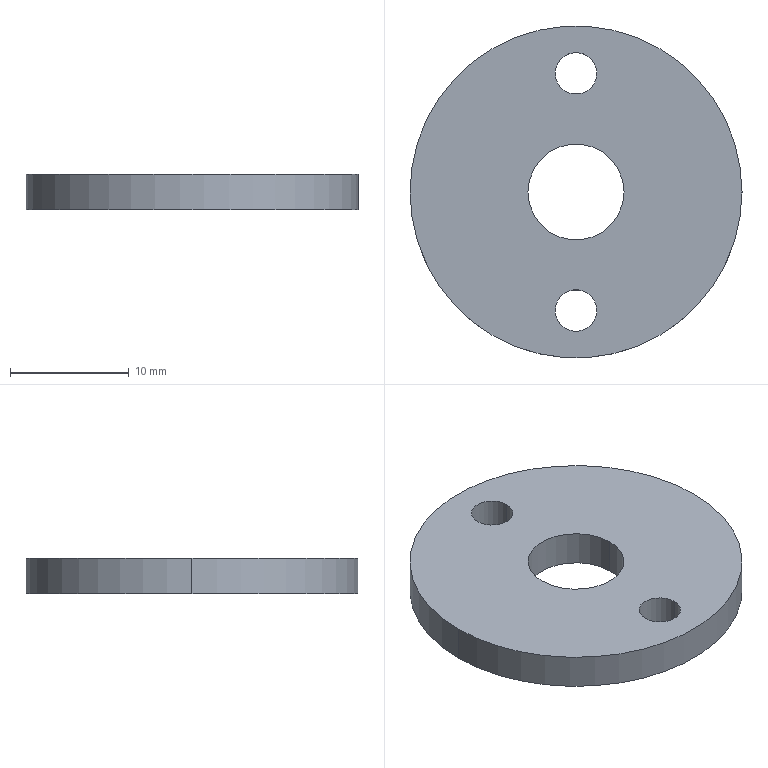Part | STEP file | BU-A19-1 | 1 solid | 10 faces | box 28 x 28 x 3 mm | volume 1635 mm3 | cylinder 8 | plane 2 | commonest cylinder face diameters 3.5 x4 8.1 x2 28 x2
STEP:
#1=CARTESIAN_POINT('',(0.,0.,0.));
#2=DIRECTION('',(0.,0.,1.));
#3=DIRECTION('',(1.,0.,0.));
#4=AXIS2_PLACEMENT_3D('',#1,#2,#3);
#5=CARTESIAN_POINT('',(-1.75,-10.,3.));
#6=VERTEX_POINT('',#5);
#7=CARTESIAN_POINT('',(-1.75,-10.,0.));
#8=VERTEX_POINT('',#7);
#9=CARTESIAN_POINT('',(-1.75,-10.,3.));
#10=DIRECTION('',(0.,0.,-1.));
#11=VECTOR('',#10,1.);
#12=LINE('',#9,#11);
#13=CARTESIAN_POINT('',(0.,-10.,3.));
#14=DIRECTION('',(0.,0.,-1.));
#15=DIRECTION('',(-1.,0.,0.));
#16=AXIS2_PLACEMENT_3D('',#13,#14,#15);
#17=CYLINDRICAL_SURFACE('',#16,1.75);
#18=CARTESIAN_POINT('',(6.283,0.));
#19=DIRECTION('',(0.,1.));
#20=VECTOR('',#19,1.);
#21=LINE('',#18,#20);
#22=(GEOMETRIC_REPRESENTATION_CONTEXT(2)PARAMETRIC_REPRESENTATION_CONTEXT()REPRESENTATION_CONTEXT('',''));
#23=DEFINITIONAL_REPRESENTATION('',(#21),#22);
#24=PCURVE('',#17,#23);
#25=CARTESIAN_POINT('',(0.,-10.,3.));
#26=DIRECTION('',(0.,0.,-1.));
#27=DIRECTION('',(-1.,0.,0.));
#28=AXIS2_PLACEMENT_3D('',#25,#26,#27);
#29=CYLINDRICAL_SURFACE('',#28,1.75);
#30=CARTESIAN_POINT('',(0.,0.));
#31=DIRECTION('',(0.,1.));
#32=VECTOR('',#31,1.);
#33=LINE('',#30,#32);
#34=(GEOMETRIC_REPRESENTATION_CONTEXT(2)PARAMETRIC_REPRESENTATION_CONTEXT()REPRESENTATION_CONTEXT('',''));
#35=DEFINITIONAL_REPRESENTATION('',(#33),#34);
#36=PCURVE('',#29,#35);
#37=SURFACE_CURVE('',#12,(#24,#36),.PCURVE_S1.);
#38=EDGE_CURVE('',#6,#8,#37,.T.);
#39=ORIENTED_EDGE('',*,*,#38,.T.);
#40=CARTESIAN_POINT('',(1.75,-10.,0.));
#41=VERTEX_POINT('',#40);
#42=CARTESIAN_POINT('',(0.,-10.,0.));
#43=DIRECTION('',(0.,0.,1.));
#44=DIRECTION('',(1.,0.,0.));
#45=AXIS2_PLACEMENT_3D('',#42,#43,#44);
#46=CIRCLE('',#45,1.75);
#47=CARTESIAN_POINT('',(9.425,3.));
#48=DIRECTION('',(-1.,0.));
#49=VECTOR('',#48,1.);
#50=LINE('',#47,#49);
#51=(GEOMETRIC_REPRESENTATION_CONTEXT(2)PARAMETRIC_REPRESENTATION_CONTEXT()REPRESENTATION_CONTEXT('',''));
#52=DEFINITIONAL_REPRESENTATION('',(#50),#51);
#53=PCURVE('',#17,#52);
#54=CARTESIAN_POINT('',(0.,0.,0.));
#55=DIRECTION('',(0.,0.,1.));
#56=DIRECTION('',(1.,0.,0.));
#57=AXIS2_PLACEMENT_3D('',#54,#55,#56);
#58=PLANE('',#57);
#59=CARTESIAN_POINT('',(0.,-10.));
#60=DIRECTION('',(1.,0.));
#61=AXIS2_PLACEMENT_2D('',#59,#60);
#62=CIRCLE('',#61,1.75);
#63=(GEOMETRIC_REPRESENTATION_CONTEXT(2)PARAMETRIC_REPRESENTATION_CONTEXT()REPRESENTATION_CONTEXT('',''));
#64=DEFINITIONAL_REPRESENTATION('',(#62),#63);
#65=PCURVE('',#58,#64);
#66=SURFACE_CURVE('',#46,(#53,#65),.PCURVE_S1.);
#67=EDGE_CURVE('',#8,#41,#66,.T.);
#68=ORIENTED_EDGE('',*,*,#67,.T.);
#69=CARTESIAN_POINT('',(1.75,-10.,3.));
#70=VERTEX_POINT('',#69);
#71=CARTESIAN_POINT('',(1.75,-10.,3.));
#72=DIRECTION('',(0.,0.,-1.));
#73=VECTOR('',#72,1.);
#74=LINE('',#71,#73);
#75=CARTESIAN_POINT('',(3.142,0.));
#76=DIRECTION('',(0.,1.));
#77=VECTOR('',#76,1.);
#78=LINE('',#75,#77);
#79=(GEOMETRIC_REPRESENTATION_CONTEXT(2)PARAMETRIC_REPRESENTATION_CONTEXT()REPRESENTATION_CONTEXT('',''));
#80=DEFINITIONAL_REPRESENTATION('',(#78),#79);
#81=PCURVE('',#17,#80);
#82=CARTESIAN_POINT('',(3.142,0.));
#83=DIRECTION('',(0.,1.));
#84=VECTOR('',#83,1.);
#85=LINE('',#82,#84);
#86=(GEOMETRIC_REPRESENTATION_CONTEXT(2)PARAMETRIC_REPRESENTATION_CONTEXT()REPRESENTATION_CONTEXT('',''));
#87=DEFINITIONAL_REPRESENTATION('',(#85),#86);
#88=PCURVE('',#29,#87);
#89=SURFACE_CURVE('',#74,(#81,#88),.PCURVE_S1.);
#90=EDGE_CURVE('',#70,#41,#89,.T.);
#91=ORIENTED_EDGE('',*,*,#90,.F.);
#92=CARTESIAN_POINT('',(0.,-10.,3.));
#93=DIRECTION('',(0.,0.,1.));
#94=DIRECTION('',(1.,0.,0.));
#95=AXIS2_PLACEMENT_3D('',#92,#93,#94);
#96=CIRCLE('',#95,1.75);
#97=CARTESIAN_POINT('',(9.425,0.));
#98=DIRECTION('',(-1.,0.));
#99=VECTOR('',#98,1.);
#100=LINE('',#97,#99);
#101=(GEOMETRIC_REPRESENTATION_CONTEXT(2)PARAMETRIC_REPRESENTATION_CONTEXT()REPRESENTATION_CONTEXT('',''));
#102=DEFINITIONAL_REPRESENTATION('',(#100),#101);
#103=PCURVE('',#17,#102);
#104=CARTESIAN_POINT('',(0.,0.,3.));
#105=DIRECTION('',(0.,0.,1.));
#106=DIRECTION('',(1.,0.,0.));
#107=AXIS2_PLACEMENT_3D('',#104,#105,#106);
#108=PLANE('',#107);
#109=CARTESIAN_POINT('',(0.,-10.));
#110=DIRECTION('',(1.,0.));
#111=AXIS2_PLACEMENT_2D('',#109,#110);
#112=CIRCLE('',#111,1.75);
#113=(GEOMETRIC_REPRESENTATION_CONTEXT(2)PARAMETRIC_REPRESENTATION_CONTEXT()REPRESENTATION_CONTEXT('',''));
#114=DEFINITIONAL_REPRESENTATION('',(#112),#113);
#115=PCURVE('',#108,#114);
#116=SURFACE_CURVE('',#96,(#103,#115),.PCURVE_S1.);
#117=EDGE_CURVE('',#6,#70,#116,.T.);
#118=ORIENTED_EDGE('',*,*,#117,.F.);
#119=EDGE_LOOP('',(#39,#68,#91,#118));
#120=FACE_BOUND('',#119,.F.);
#121=ADVANCED_FACE('',(#120),#17,.F.);
#122=CARTESIAN_POINT('',(-1.75,10.,3.));
#123=VERTEX_POINT('',#122);
#124=CARTESIAN_POINT('',(-1.75,10.,0.));
#125=VERTEX_POINT('',#124);
#126=CARTESIAN_POINT('',(-1.75,10.,3.));
#127=DIRECTION('',(0.,0.,-1.));
#128=VECTOR('',#127,1.);
#129=LINE('',#126,#128);
#130=CARTESIAN_POINT('',(0.,10.,3.));
#131=DIRECTION('',(0.,0.,-1.));
#132=DIRECTION('',(-1.,0.,0.));
#133=AXIS2_PLACEMENT_3D('',#130,#131,#132);
#134=CYLINDRICAL_SURFACE('',#133,1.75);
#135=CARTESIAN_POINT('',(6.283,0.));
#136=DIRECTION('',(0.,1.));
#137=VECTOR('',#136,1.);
#138=LINE('',#135,#137);
#139=(GEOMETRIC_REPRESENTATION_CONTEXT(2)PARAMETRIC_REPRESENTATION_CONTEXT()REPRESENTATION_CONTEXT('',''));
#140=DEFINITIONAL_REPRESENTATION('',(#138),#139);
#141=PCURVE('',#134,#140);
#142=CARTESIAN_POINT('',(0.,10.,3.));
#143=DIRECTION('',(0.,0.,-1.));
#144=DIRECTION('',(-1.,0.,0.));
#145=AXIS2_PLACEMENT_3D('',#142,#143,#144);
#146=CYLINDRICAL_SURFACE('',#145,1.75);
#147=CARTESIAN_POINT('',(0.,0.));
#148=DIRECTION('',(0.,1.));
#149=VECTOR('',#148,1.);
#150=LINE('',#147,#149);
#151=(GEOMETRIC_REPRESENTATION_CONTEXT(2)PARAMETRIC_REPRESENTATION_CONTEXT()REPRESENTATION_CONTEXT('',''));
#152=DEFINITIONAL_REPRESENTATION('',(#150),#151);
#153=PCURVE('',#146,#152);
#154=SURFACE_CURVE('',#129,(#141,#153),.PCURVE_S1.);
#155=EDGE_CURVE('',#123,#125,#154,.T.);
#156=ORIENTED_EDGE('',*,*,#155,.T.);
#157=CARTESIAN_POINT('',(1.75,10.,0.));
#158=VERTEX_POINT('',#157);
#159=CARTESIAN_POINT('',(0.,10.,0.));
#160=DIRECTION('',(0.,0.,1.));
#161=DIRECTION('',(1.,0.,0.));
#162=AXIS2_PLACEMENT_3D('',#159,#160,#161);
#163=CIRCLE('',#162,1.75);
#164=CARTESIAN_POINT('',(9.425,3.));
#165=DIRECTION('',(-1.,0.));
#166=VECTOR('',#165,1.);
#167=LINE('',#164,#166);
#168=(GEOMETRIC_REPRESENTATION_CONTEXT(2)PARAMETRIC_REPRESENTATION_CONTEXT()REPRESENTATION_CONTEXT('',''));
#169=DEFINITIONAL_REPRESENTATION('',(#167),#168);
#170=PCURVE('',#134,#169);
#171=CARTESIAN_POINT('',(0.,10.));
#172=DIRECTION('',(1.,0.));
#173=AXIS2_PLACEMENT_2D('',#171,#172);
#174=CIRCLE('',#173,1.75);
#175=(GEOMETRIC_REPRESENTATION_CONTEXT(2)PARAMETRIC_REPRESENTATION_CONTEXT()REPRESENTATION_CONTEXT('',''));
#176=DEFINITIONAL_REPRESENTATION('',(#174),#175);
#177=PCURVE('',#58,#176);
#178=SURFACE_CURVE('',#163,(#170,#177),.PCURVE_S1.);
#179=EDGE_CURVE('',#125,#158,#178,.T.);
#180=ORIENTED_EDGE('',*,*,#179,.T.);
#181=CARTESIAN_POINT('',(1.75,10.,3.));
#182=VERTEX_POINT('',#181);
#183=CARTESIAN_POINT('',(1.75,10.,3.));
#184=DIRECTION('',(0.,0.,-1.));
#185=VECTOR('',#184,1.);
#186=LINE('',#183,#185);
#187=CARTESIAN_POINT('',(3.142,0.));
#188=DIRECTION('',(0.,1.));
#189=VECTOR('',#188,1.);
#190=LINE('',#187,#189);
#191=(GEOMETRIC_REPRESENTATION_CONTEXT(2)PARAMETRIC_REPRESENTATION_CONTEXT()REPRESENTATION_CONTEXT('',''));
#192=DEFINITIONAL_REPRESENTATION('',(#190),#191);
#193=PCURVE('',#134,#192);
#194=CARTESIAN_POINT('',(3.142,0.));
#195=DIRECTION('',(0.,1.));
#196=VECTOR('',#195,1.);
#197=LINE('',#194,#196);
#198=(GEOMETRIC_REPRESENTATION_CONTEXT(2)PARAMETRIC_REPRESENTATION_CONTEXT()REPRESENTATION_CONTEXT('',''));
#199=DEFINITIONAL_REPRESENTATION('',(#197),#198);
#200=PCURVE('',#146,#199);
#201=SURFACE_CURVE('',#186,(#193,#200),.PCURVE_S1.);
#202=EDGE_CURVE('',#182,#158,#201,.T.);
#203=ORIENTED_EDGE('',*,*,#202,.F.);
#204=CARTESIAN_POINT('',(0.,10.,3.));
#205=DIRECTION('',(0.,0.,1.));
#206=DIRECTION('',(1.,0.,0.));
#207=AXIS2_PLACEMENT_3D('',#204,#205,#206);
#208=CIRCLE('',#207,1.75);
#209=CARTESIAN_POINT('',(9.425,0.));
#210=DIRECTION('',(-1.,0.));
#211=VECTOR('',#210,1.);
#212=LINE('',#209,#211);
#213=(GEOMETRIC_REPRESENTATION_CONTEXT(2)PARAMETRIC_REPRESENTATION_CONTEXT()REPRESENTATION_CONTEXT('',''));
#214=DEFINITIONAL_REPRESENTATION('',(#212),#213);
#215=PCURVE('',#134,#214);
#216=CARTESIAN_POINT('',(0.,10.));
#217=DIRECTION('',(1.,0.));
#218=AXIS2_PLACEMENT_2D('',#216,#217);
#219=CIRCLE('',#218,1.75);
#220=(GEOMETRIC_REPRESENTATION_CONTEXT(2)PARAMETRIC_REPRESENTATION_CONTEXT()REPRESENTATION_CONTEXT('',''));
#221=DEFINITIONAL_REPRESENTATION('',(#219),#220);
#222=PCURVE('',#108,#221);
#223=SURFACE_CURVE('',#208,(#215,#222),.PCURVE_S1.);
#224=EDGE_CURVE('',#123,#182,#223,.T.);
#225=ORIENTED_EDGE('',*,*,#224,.F.);
#226=EDGE_LOOP('',(#156,#180,#203,#225));
#227=FACE_BOUND('',#226,.F.);
#228=ADVANCED_FACE('',(#227),#134,.F.);
#229=CARTESIAN_POINT('',(-4.05,0.,3.));
#230=VERTEX_POINT('',#229);
#231=CARTESIAN_POINT('',(-4.05,0.,0.));
#232=VERTEX_POINT('',#231);
#233=CARTESIAN_POINT('',(-4.05,0.,3.));
#234=DIRECTION('',(0.,0.,-1.));
#235=VECTOR('',#234,1.);
#236=LINE('',#233,#235);
#237=CARTESIAN_POINT('',(0.,0.,3.));
#238=DIRECTION('',(0.,0.,-1.));
#239=DIRECTION('',(-1.,0.,0.));
#240=AXIS2_PLACEMENT_3D('',#237,#238,#239);
#241=CYLINDRICAL_SURFACE('',#240,4.05);
#242=CARTESIAN_POINT('',(6.283,0.));
#243=DIRECTION('',(0.,1.));
#244=VECTOR('',#243,1.);
#245=LINE('',#242,#244);
#246=(GEOMETRIC_REPRESENTATION_CONTEXT(2)PARAMETRIC_REPRESENTATION_CONTEXT()REPRESENTATION_CONTEXT('',''));
#247=DEFINITIONAL_REPRESENTATION('',(#245),#246);
#248=PCURVE('',#241,#247);
#249=CARTESIAN_POINT('',(0.,0.,3.));
#250=DIRECTION('',(0.,0.,-1.));
#251=DIRECTION('',(-1.,0.,0.));
#252=AXIS2_PLACEMENT_3D('',#249,#250,#251);
#253=CYLINDRICAL_SURFACE('',#252,4.05);
#254=CARTESIAN_POINT('',(0.,0.));
#255=DIRECTION('',(0.,1.));
#256=VECTOR('',#255,1.);
#257=LINE('',#254,#256);
#258=(GEOMETRIC_REPRESENTATION_CONTEXT(2)PARAMETRIC_REPRESENTATION_CONTEXT()REPRESENTATION_CONTEXT('',''));
#259=DEFINITIONAL_REPRESENTATION('',(#257),#258);
#260=PCURVE('',#253,#259);
#261=SURFACE_CURVE('',#236,(#248,#260),.PCURVE_S1.);
#262=EDGE_CURVE('',#230,#232,#261,.T.);
#263=ORIENTED_EDGE('',*,*,#262,.T.);
#264=CARTESIAN_POINT('',(4.05,0.,0.));
#265=VERTEX_POINT('',#264);
#266=CARTESIAN_POINT('',(0.,0.,0.));
#267=DIRECTION('',(0.,0.,1.));
#268=DIRECTION('',(1.,0.,0.));
#269=AXIS2_PLACEMENT_3D('',#266,#267,#268);
#270=CIRCLE('',#269,4.05);
#271=CARTESIAN_POINT('',(9.425,3.));
#272=DIRECTION('',(-1.,0.));
#273=VECTOR('',#272,1.);
#274=LINE('',#271,#273);
#275=(GEOMETRIC_REPRESENTATION_CONTEXT(2)PARAMETRIC_REPRESENTATION_CONTEXT()REPRESENTATION_CONTEXT('',''));
#276=DEFINITIONAL_REPRESENTATION('',(#274),#275);
#277=PCURVE('',#241,#276);
#278=CARTESIAN_POINT('',(0.,0.));
#279=DIRECTION('',(1.,0.));
#280=AXIS2_PLACEMENT_2D('',#278,#279);
#281=CIRCLE('',#280,4.05);
#282=(GEOMETRIC_REPRESENTATION_CONTEXT(2)PARAMETRIC_REPRESENTATION_CONTEXT()REPRESENTATION_CONTEXT('',''));
#283=DEFINITIONAL_REPRESENTATION('',(#281),#282);
#284=PCURVE('',#58,#283);
#285=SURFACE_CURVE('',#270,(#277,#284),.PCURVE_S1.);
#286=EDGE_CURVE('',#232,#265,#285,.T.);
#287=ORIENTED_EDGE('',*,*,#286,.T.);
#288=CARTESIAN_POINT('',(4.05,0.,3.));
#289=VERTEX_POINT('',#288);
#290=CARTESIAN_POINT('',(4.05,0.,3.));
#291=DIRECTION('',(0.,0.,-1.));
#292=VECTOR('',#291,1.);
#293=LINE('',#290,#292);
#294=CARTESIAN_POINT('',(3.142,0.));
#295=DIRECTION('',(0.,1.));
#296=VECTOR('',#295,1.);
#297=LINE('',#294,#296);
#298=(GEOMETRIC_REPRESENTATION_CONTEXT(2)PARAMETRIC_REPRESENTATION_CONTEXT()REPRESENTATION_CONTEXT('',''));
#299=DEFINITIONAL_REPRESENTATION('',(#297),#298);
#300=PCURVE('',#241,#299);
#301=CARTESIAN_POINT('',(3.142,0.));
#302=DIRECTION('',(0.,1.));
#303=VECTOR('',#302,1.);
#304=LINE('',#301,#303);
#305=(GEOMETRIC_REPRESENTATION_CONTEXT(2)PARAMETRIC_REPRESENTATION_CONTEXT()REPRESENTATION_CONTEXT('',''));
#306=DEFINITIONAL_REPRESENTATION('',(#304),#305);
#307=PCURVE('',#253,#306);
#308=SURFACE_CURVE('',#293,(#300,#307),.PCURVE_S1.);
#309=EDGE_CURVE('',#289,#265,#308,.T.);
#310=ORIENTED_EDGE('',*,*,#309,.F.);
#311=CARTESIAN_POINT('',(0.,0.,3.));
#312=DIRECTION('',(0.,0.,1.));
#313=DIRECTION('',(1.,0.,0.));
#314=AXIS2_PLACEMENT_3D('',#311,#312,#313);
#315=CIRCLE('',#314,4.05);
#316=CARTESIAN_POINT('',(9.425,0.));
#317=DIRECTION('',(-1.,0.));
#318=VECTOR('',#317,1.);
#319=LINE('',#316,#318);
#320=(GEOMETRIC_REPRESENTATION_CONTEXT(2)PARAMETRIC_REPRESENTATION_CONTEXT()REPRESENTATION_CONTEXT('',''));
#321=DEFINITIONAL_REPRESENTATION('',(#319),#320);
#322=PCURVE('',#241,#321);
#323=CARTESIAN_POINT('',(0.,0.));
#324=DIRECTION('',(1.,0.));
#325=AXIS2_PLACEMENT_2D('',#323,#324);
#326=CIRCLE('',#325,4.05);
#327=(GEOMETRIC_REPRESENTATION_CONTEXT(2)PARAMETRIC_REPRESENTATION_CONTEXT()REPRESENTATION_CONTEXT('',''));
#328=DEFINITIONAL_REPRESENTATION('',(#326),#327);
#329=PCURVE('',#108,#328);
#330=SURFACE_CURVE('',#315,(#322,#329),.PCURVE_S1.);
#331=EDGE_CURVE('',#230,#289,#330,.T.);
#332=ORIENTED_EDGE('',*,*,#331,.F.);
#333=EDGE_LOOP('',(#263,#287,#310,#332));
#334=FACE_BOUND('',#333,.F.);
#335=ADVANCED_FACE('',(#334),#241,.F.);
#336=CARTESIAN_POINT('',(14.,0.,3.));
#337=VERTEX_POINT('',#336);
#338=CARTESIAN_POINT('',(-14.,0.,3.));
#339=VERTEX_POINT('',#338);
#340=CARTESIAN_POINT('',(0.,0.,3.));
#341=DIRECTION('',(0.,0.,1.));
#342=DIRECTION('',(1.,0.,0.));
#343=AXIS2_PLACEMENT_3D('',#340,#341,#342);
#344=CIRCLE('',#343,14.);
#345=CARTESIAN_POINT('',(0.,0.,3.));
#346=DIRECTION('',(0.,0.,-1.));
#347=DIRECTION('',(-1.,0.,0.));
#348=AXIS2_PLACEMENT_3D('',#345,#346,#347);
#349=CYLINDRICAL_SURFACE('',#348,14.);
#350=CARTESIAN_POINT('',(3.142,0.));
#351=DIRECTION('',(-1.,0.));
#352=VECTOR('',#351,1.);
#353=LINE('',#350,#352);
#354=(GEOMETRIC_REPRESENTATION_CONTEXT(2)PARAMETRIC_REPRESENTATION_CONTEXT()REPRESENTATION_CONTEXT('',''));
#355=DEFINITIONAL_REPRESENTATION('',(#353),#354);
#356=PCURVE('',#349,#355);
#357=CARTESIAN_POINT('',(0.,0.));
#358=DIRECTION('',(1.,0.));
#359=AXIS2_PLACEMENT_2D('',#357,#358);
#360=CIRCLE('',#359,14.);
#361=(GEOMETRIC_REPRESENTATION_CONTEXT(2)PARAMETRIC_REPRESENTATION_CONTEXT()REPRESENTATION_CONTEXT('',''));
#362=DEFINITIONAL_REPRESENTATION('',(#360),#361);
#363=PCURVE('',#108,#362);
#364=SURFACE_CURVE('',#344,(#356,#363),.PCURVE_S1.);
#365=EDGE_CURVE('',#337,#339,#364,.T.);
#366=ORIENTED_EDGE('',*,*,#365,.F.);
#367=CARTESIAN_POINT('',(14.,0.,0.));
#368=VERTEX_POINT('',#367);
#369=CARTESIAN_POINT('',(14.,0.,3.));
#370=DIRECTION('',(0.,0.,-1.));
#371=VECTOR('',#370,1.);
#372=LINE('',#369,#371);
#373=CARTESIAN_POINT('',(3.142,0.));
#374=DIRECTION('',(0.,1.));
#375=VECTOR('',#374,1.);
#376=LINE('',#373,#375);
#377=(GEOMETRIC_REPRESENTATION_CONTEXT(2)PARAMETRIC_REPRESENTATION_CONTEXT()REPRESENTATION_CONTEXT('',''));
#378=DEFINITIONAL_REPRESENTATION('',(#376),#377);
#379=PCURVE('',#349,#378);
#380=CARTESIAN_POINT('',(0.,0.,3.));
#381=DIRECTION('',(0.,0.,-1.));
#382=DIRECTION('',(-1.,0.,0.));
#383=AXIS2_PLACEMENT_3D('',#380,#381,#382);
#384=CYLINDRICAL_SURFACE('',#383,14.);
#385=CARTESIAN_POINT('',(3.142,0.));
#386=DIRECTION('',(0.,1.));
#387=VECTOR('',#386,1.);
#388=LINE('',#385,#387);
#389=(GEOMETRIC_REPRESENTATION_CONTEXT(2)PARAMETRIC_REPRESENTATION_CONTEXT()REPRESENTATION_CONTEXT('',''));
#390=DEFINITIONAL_REPRESENTATION('',(#388),#389);
#391=PCURVE('',#384,#390);
#392=SURFACE_CURVE('',#372,(#379,#391),.PCURVE_S1.);
#393=EDGE_CURVE('',#337,#368,#392,.T.);
#394=ORIENTED_EDGE('',*,*,#393,.T.);
#395=CARTESIAN_POINT('',(-14.,0.,0.));
#396=VERTEX_POINT('',#395);
#397=CARTESIAN_POINT('',(0.,0.,0.));
#398=DIRECTION('',(0.,0.,1.));
#399=DIRECTION('',(1.,0.,0.));
#400=AXIS2_PLACEMENT_3D('',#397,#398,#399);
#401=CIRCLE('',#400,14.);
#402=CARTESIAN_POINT('',(3.142,3.));
#403=DIRECTION('',(-1.,0.));
#404=VECTOR('',#403,1.);
#405=LINE('',#402,#404);
#406=(GEOMETRIC_REPRESENTATION_CONTEXT(2)PARAMETRIC_REPRESENTATION_CONTEXT()REPRESENTATION_CONTEXT('',''));
#407=DEFINITIONAL_REPRESENTATION('',(#405),#406);
#408=PCURVE('',#349,#407);
#409=CARTESIAN_POINT('',(0.,0.));
#410=DIRECTION('',(1.,0.));
#411=AXIS2_PLACEMENT_2D('',#409,#410);
#412=CIRCLE('',#411,14.);
#413=(GEOMETRIC_REPRESENTATION_CONTEXT(2)PARAMETRIC_REPRESENTATION_CONTEXT()REPRESENTATION_CONTEXT('',''));
#414=DEFINITIONAL_REPRESENTATION('',(#412),#413);
#415=PCURVE('',#58,#414);
#416=SURFACE_CURVE('',#401,(#408,#415),.PCURVE_S1.);
#417=EDGE_CURVE('',#368,#396,#416,.T.);
#418=ORIENTED_EDGE('',*,*,#417,.T.);
#419=CARTESIAN_POINT('',(-14.,0.,3.));
#420=DIRECTION('',(0.,0.,-1.));
#421=VECTOR('',#420,1.);
#422=LINE('',#419,#421);
#423=CARTESIAN_POINT('',(0.,0.));
#424=DIRECTION('',(0.,1.));
#425=VECTOR('',#424,1.);
#426=LINE('',#423,#425);
#427=(GEOMETRIC_REPRESENTATION_CONTEXT(2)PARAMETRIC_REPRESENTATION_CONTEXT()REPRESENTATION_CONTEXT('',''));
#428=DEFINITIONAL_REPRESENTATION('',(#426),#427);
#429=PCURVE('',#349,#428);
#430=CARTESIAN_POINT('',(6.283,0.));
#431=DIRECTION('',(0.,1.));
#432=VECTOR('',#431,1.);
#433=LINE('',#430,#432);
#434=(GEOMETRIC_REPRESENTATION_CONTEXT(2)PARAMETRIC_REPRESENTATION_CONTEXT()REPRESENTATION_CONTEXT('',''));
#435=DEFINITIONAL_REPRESENTATION('',(#433),#434);
#436=PCURVE('',#384,#435);
#437=SURFACE_CURVE('',#422,(#429,#436),.PCURVE_S1.);
#438=EDGE_CURVE('',#339,#396,#437,.T.);
#439=ORIENTED_EDGE('',*,*,#438,.F.);
#440=EDGE_LOOP('',(#366,#394,#418,#439));
#441=FACE_BOUND('',#440,.T.);
#442=ADVANCED_FACE('',(#441),#349,.T.);
#443=ORIENTED_EDGE('',*,*,#224,.F.);
#444=CARTESIAN_POINT('',(0.,10.,3.));
#445=DIRECTION('',(0.,0.,1.));
#446=DIRECTION('',(1.,0.,0.));
#447=AXIS2_PLACEMENT_3D('',#444,#445,#446);
#448=CIRCLE('',#447,1.75);
#449=CARTESIAN_POINT('',(0.,10.));
#450=DIRECTION('',(1.,0.));
#451=AXIS2_PLACEMENT_2D('',#449,#450);
#452=CIRCLE('',#451,1.75);
#453=(GEOMETRIC_REPRESENTATION_CONTEXT(2)PARAMETRIC_REPRESENTATION_CONTEXT()REPRESENTATION_CONTEXT('',''));
#454=DEFINITIONAL_REPRESENTATION('',(#452),#453);
#455=PCURVE('',#108,#454);
#456=CARTESIAN_POINT('',(3.142,0.));
#457=DIRECTION('',(-1.,0.));
#458=VECTOR('',#457,1.);
#459=LINE('',#456,#458);
#460=(GEOMETRIC_REPRESENTATION_CONTEXT(2)PARAMETRIC_REPRESENTATION_CONTEXT()REPRESENTATION_CONTEXT('',''));
#461=DEFINITIONAL_REPRESENTATION('',(#459),#460);
#462=PCURVE('',#146,#461);
#463=SURFACE_CURVE('',#448,(#455,#462),.PCURVE_S1.);
#464=EDGE_CURVE('',#182,#123,#463,.T.);
#465=ORIENTED_EDGE('',*,*,#464,.F.);
#466=EDGE_LOOP('',(#443,#465));
#467=FACE_BOUND('',#466,.T.);
#468=CARTESIAN_POINT('',(0.,0.,3.));
#469=DIRECTION('',(0.,0.,1.));
#470=DIRECTION('',(1.,0.,0.));
#471=AXIS2_PLACEMENT_3D('',#468,#469,#470);
#472=CIRCLE('',#471,14.);
#473=CARTESIAN_POINT('',(0.,0.));
#474=DIRECTION('',(1.,0.));
#475=AXIS2_PLACEMENT_2D('',#473,#474);
#476=CIRCLE('',#475,14.);
#477=(GEOMETRIC_REPRESENTATION_CONTEXT(2)PARAMETRIC_REPRESENTATION_CONTEXT()REPRESENTATION_CONTEXT('',''));
#478=DEFINITIONAL_REPRESENTATION('',(#476),#477);
#479=PCURVE('',#108,#478);
#480=CARTESIAN_POINT('',(9.425,0.));
#481=DIRECTION('',(-1.,0.));
#482=VECTOR('',#481,1.);
#483=LINE('',#480,#482);
#484=(GEOMETRIC_REPRESENTATION_CONTEXT(2)PARAMETRIC_REPRESENTATION_CONTEXT()REPRESENTATION_CONTEXT('',''));
#485=DEFINITIONAL_REPRESENTATION('',(#483),#484);
#486=PCURVE('',#384,#485);
#487=SURFACE_CURVE('',#472,(#479,#486),.PCURVE_S1.);
#488=EDGE_CURVE('',#339,#337,#487,.T.);
#489=ORIENTED_EDGE('',*,*,#488,.T.);
#490=ORIENTED_EDGE('',*,*,#365,.T.);
#491=EDGE_LOOP('',(#489,#490));
#492=FACE_BOUND('',#491,.T.);
#493=ORIENTED_EDGE('',*,*,#331,.F.);
#494=CARTESIAN_POINT('',(0.,0.,3.));
#495=DIRECTION('',(0.,0.,1.));
#496=DIRECTION('',(1.,0.,0.));
#497=AXIS2_PLACEMENT_3D('',#494,#495,#496);
#498=CIRCLE('',#497,4.05);
#499=CARTESIAN_POINT('',(0.,0.));
#500=DIRECTION('',(1.,0.));
#501=AXIS2_PLACEMENT_2D('',#499,#500);
#502=CIRCLE('',#501,4.05);
#503=(GEOMETRIC_REPRESENTATION_CONTEXT(2)PARAMETRIC_REPRESENTATION_CONTEXT()REPRESENTATION_CONTEXT('',''));
#504=DEFINITIONAL_REPRESENTATION('',(#502),#503);
#505=PCURVE('',#108,#504);
#506=CARTESIAN_POINT('',(3.142,0.));
#507=DIRECTION('',(-1.,0.));
#508=VECTOR('',#507,1.);
#509=LINE('',#506,#508);
#510=(GEOMETRIC_REPRESENTATION_CONTEXT(2)PARAMETRIC_REPRESENTATION_CONTEXT()REPRESENTATION_CONTEXT('',''));
#511=DEFINITIONAL_REPRESENTATION('',(#509),#510);
#512=PCURVE('',#253,#511);
#513=SURFACE_CURVE('',#498,(#505,#512),.PCURVE_S1.);
#514=EDGE_CURVE('',#289,#230,#513,.T.);
#515=ORIENTED_EDGE('',*,*,#514,.F.);
#516=EDGE_LOOP('',(#493,#515));
#517=FACE_BOUND('',#516,.T.);
#518=ORIENTED_EDGE('',*,*,#117,.F.);
#519=CARTESIAN_POINT('',(0.,-10.,3.));
#520=DIRECTION('',(0.,0.,1.));
#521=DIRECTION('',(1.,0.,0.));
#522=AXIS2_PLACEMENT_3D('',#519,#520,#521);
#523=CIRCLE('',#522,1.75);
#524=CARTESIAN_POINT('',(0.,-10.));
#525=DIRECTION('',(1.,0.));
#526=AXIS2_PLACEMENT_2D('',#524,#525);
#527=CIRCLE('',#526,1.75);
#528=(GEOMETRIC_REPRESENTATION_CONTEXT(2)PARAMETRIC_REPRESENTATION_CONTEXT()REPRESENTATION_CONTEXT('',''));
#529=DEFINITIONAL_REPRESENTATION('',(#527),#528);
#530=PCURVE('',#108,#529);
#531=CARTESIAN_POINT('',(3.142,0.));
#532=DIRECTION('',(-1.,0.));
#533=VECTOR('',#532,1.);
#534=LINE('',#531,#533);
#535=(GEOMETRIC_REPRESENTATION_CONTEXT(2)PARAMETRIC_REPRESENTATION_CONTEXT()REPRESENTATION_CONTEXT('',''));
#536=DEFINITIONAL_REPRESENTATION('',(#534),#535);
#537=PCURVE('',#29,#536);
#538=SURFACE_CURVE('',#523,(#530,#537),.PCURVE_S1.);
#539=EDGE_CURVE('',#70,#6,#538,.T.);
#540=ORIENTED_EDGE('',*,*,#539,.F.);
#541=EDGE_LOOP('',(#518,#540));
#542=FACE_BOUND('',#541,.T.);
#543=ADVANCED_FACE('',(#467,#492,#517,#542),#108,.T.);
#544=ORIENTED_EDGE('',*,*,#179,.T.);
#545=CARTESIAN_POINT('',(0.,10.,0.));
#546=DIRECTION('',(0.,0.,1.));
#547=DIRECTION('',(1.,0.,0.));
#548=AXIS2_PLACEMENT_3D('',#545,#546,#547);
#549=CIRCLE('',#548,1.75);
#550=CARTESIAN_POINT('',(0.,10.));
#551=DIRECTION('',(1.,0.));
#552=AXIS2_PLACEMENT_2D('',#550,#551);
#553=CIRCLE('',#552,1.75);
#554=(GEOMETRIC_REPRESENTATION_CONTEXT(2)PARAMETRIC_REPRESENTATION_CONTEXT()REPRESENTATION_CONTEXT('',''));
#555=DEFINITIONAL_REPRESENTATION('',(#553),#554);
#556=PCURVE('',#58,#555);
#557=CARTESIAN_POINT('',(3.142,3.));
#558=DIRECTION('',(-1.,0.));
#559=VECTOR('',#558,1.);
#560=LINE('',#557,#559);
#561=(GEOMETRIC_REPRESENTATION_CONTEXT(2)PARAMETRIC_REPRESENTATION_CONTEXT()REPRESENTATION_CONTEXT('',''));
#562=DEFINITIONAL_REPRESENTATION('',(#560),#561);
#563=PCURVE('',#146,#562);
#564=SURFACE_CURVE('',#549,(#556,#563),.PCURVE_S1.);
#565=EDGE_CURVE('',#158,#125,#564,.T.);
#566=ORIENTED_EDGE('',*,*,#565,.T.);
#567=EDGE_LOOP('',(#544,#566));
#568=FACE_BOUND('',#567,.T.);
#569=CARTESIAN_POINT('',(0.,0.,0.));
#570=DIRECTION('',(0.,0.,1.));
#571=DIRECTION('',(1.,0.,0.));
#572=AXIS2_PLACEMENT_3D('',#569,#570,#571);
#573=CIRCLE('',#572,14.);
#574=CARTESIAN_POINT('',(0.,0.));
#575=DIRECTION('',(1.,0.));
#576=AXIS2_PLACEMENT_2D('',#574,#575);
#577=CIRCLE('',#576,14.);
#578=(GEOMETRIC_REPRESENTATION_CONTEXT(2)PARAMETRIC_REPRESENTATION_CONTEXT()REPRESENTATION_CONTEXT('',''));
#579=DEFINITIONAL_REPRESENTATION('',(#577),#578);
#580=PCURVE('',#58,#579);
#581=CARTESIAN_POINT('',(9.425,3.));
#582=DIRECTION('',(-1.,0.));
#583=VECTOR('',#582,1.);
#584=LINE('',#581,#583);
#585=(GEOMETRIC_REPRESENTATION_CONTEXT(2)PARAMETRIC_REPRESENTATION_CONTEXT()REPRESENTATION_CONTEXT('',''));
#586=DEFINITIONAL_REPRESENTATION('',(#584),#585);
#587=PCURVE('',#384,#586);
#588=SURFACE_CURVE('',#573,(#580,#587),.PCURVE_S1.);
#589=EDGE_CURVE('',#396,#368,#588,.T.);
#590=ORIENTED_EDGE('',*,*,#589,.F.);
#591=ORIENTED_EDGE('',*,*,#417,.F.);
#592=EDGE_LOOP('',(#590,#591));
#593=FACE_BOUND('',#592,.T.);
#594=ORIENTED_EDGE('',*,*,#286,.T.);
#595=CARTESIAN_POINT('',(0.,0.,0.));
#596=DIRECTION('',(0.,0.,1.));
#597=DIRECTION('',(1.,0.,0.));
#598=AXIS2_PLACEMENT_3D('',#595,#596,#597);
#599=CIRCLE('',#598,4.05);
#600=CARTESIAN_POINT('',(0.,0.));
#601=DIRECTION('',(1.,0.));
#602=AXIS2_PLACEMENT_2D('',#600,#601);
#603=CIRCLE('',#602,4.05);
#604=(GEOMETRIC_REPRESENTATION_CONTEXT(2)PARAMETRIC_REPRESENTATION_CONTEXT()REPRESENTATION_CONTEXT('',''));
#605=DEFINITIONAL_REPRESENTATION('',(#603),#604);
#606=PCURVE('',#58,#605);
#607=CARTESIAN_POINT('',(3.142,3.));
#608=DIRECTION('',(-1.,0.));
#609=VECTOR('',#608,1.);
#610=LINE('',#607,#609);
#611=(GEOMETRIC_REPRESENTATION_CONTEXT(2)PARAMETRIC_REPRESENTATION_CONTEXT()REPRESENTATION_CONTEXT('',''));
#612=DEFINITIONAL_REPRESENTATION('',(#610),#611);
#613=PCURVE('',#253,#612);
#614=SURFACE_CURVE('',#599,(#606,#613),.PCURVE_S1.);
#615=EDGE_CURVE('',#265,#232,#614,.T.);
#616=ORIENTED_EDGE('',*,*,#615,.T.);
#617=EDGE_LOOP('',(#594,#616));
#618=FACE_BOUND('',#617,.T.);
#619=ORIENTED_EDGE('',*,*,#67,.T.);
#620=CARTESIAN_POINT('',(0.,-10.,0.));
#621=DIRECTION('',(0.,0.,1.));
#622=DIRECTION('',(1.,0.,0.));
#623=AXIS2_PLACEMENT_3D('',#620,#621,#622);
#624=CIRCLE('',#623,1.75);
#625=CARTESIAN_POINT('',(0.,-10.));
#626=DIRECTION('',(1.,0.));
#627=AXIS2_PLACEMENT_2D('',#625,#626);
#628=CIRCLE('',#627,1.75);
#629=(GEOMETRIC_REPRESENTATION_CONTEXT(2)PARAMETRIC_REPRESENTATION_CONTEXT()REPRESENTATION_CONTEXT('',''));
#630=DEFINITIONAL_REPRESENTATION('',(#628),#629);
#631=PCURVE('',#58,#630);
#632=CARTESIAN_POINT('',(3.142,3.));
#633=DIRECTION('',(-1.,0.));
#634=VECTOR('',#633,1.);
#635=LINE('',#632,#634);
#636=(GEOMETRIC_REPRESENTATION_CONTEXT(2)PARAMETRIC_REPRESENTATION_CONTEXT()REPRESENTATION_CONTEXT('',''));
#637=DEFINITIONAL_REPRESENTATION('',(#635),#636);
#638=PCURVE('',#29,#637);
#639=SURFACE_CURVE('',#624,(#631,#638),.PCURVE_S1.);
#640=EDGE_CURVE('',#41,#8,#639,.T.);
#641=ORIENTED_EDGE('',*,*,#640,.T.);
#642=EDGE_LOOP('',(#619,#641));
#643=FACE_BOUND('',#642,.T.);
#644=ADVANCED_FACE('',(#568,#593,#618,#643),#58,.F.);
#645=ORIENTED_EDGE('',*,*,#393,.F.);
#646=ORIENTED_EDGE('',*,*,#488,.F.);
#647=ORIENTED_EDGE('',*,*,#438,.T.);
#648=ORIENTED_EDGE('',*,*,#589,.T.);
#649=EDGE_LOOP('',(#645,#646,#647,#648));
#650=FACE_BOUND('',#649,.T.);
#651=ADVANCED_FACE('',(#650),#384,.T.);
#652=ORIENTED_EDGE('',*,*,#615,.T.);
#653=ORIENTED_EDGE('',*,*,#262,.F.);
#654=ORIENTED_EDGE('',*,*,#514,.F.);
#655=ORIENTED_EDGE('',*,*,#309,.T.);
#656=EDGE_LOOP('',(#652,#653,#654,#655));
#657=FACE_BOUND('',#656,.F.);
#658=ADVANCED_FACE('',(#657),#253,.F.);
#659=ORIENTED_EDGE('',*,*,#565,.T.);
#660=ORIENTED_EDGE('',*,*,#155,.F.);
#661=ORIENTED_EDGE('',*,*,#464,.F.);
#662=ORIENTED_EDGE('',*,*,#202,.T.);
#663=EDGE_LOOP('',(#659,#660,#661,#662));
#664=FACE_BOUND('',#663,.F.);
#665=ADVANCED_FACE('',(#664),#146,.F.);
#666=ORIENTED_EDGE('',*,*,#640,.T.);
#667=ORIENTED_EDGE('',*,*,#38,.F.);
#668=ORIENTED_EDGE('',*,*,#539,.F.);
#669=ORIENTED_EDGE('',*,*,#90,.T.);
#670=EDGE_LOOP('',(#666,#667,#668,#669));
#671=FACE_BOUND('',#670,.F.);
#672=ADVANCED_FACE('',(#671),#29,.F.);
#673=CLOSED_SHELL('',(#121,#228,#335,#442,#543,#644,#651,#658,#665,#672));
#674=MANIFOLD_SOLID_BREP('',#673);
#675=(LENGTH_UNIT()NAMED_UNIT(*)SI_UNIT(.MILLI.,.METRE.));
#676=UNCERTAINTY_MEASURE_WITH_UNIT(LENGTH_MEASURE(0.0000001),#675,'','');
#677=(NAMED_UNIT(*)PLANE_ANGLE_UNIT()SI_UNIT($,.RADIAN.));
#678=(NAMED_UNIT(*)SI_UNIT($,.STERADIAN.)SOLID_ANGLE_UNIT());
#679=(GEOMETRIC_REPRESENTATION_CONTEXT(3)GLOBAL_UNCERTAINTY_ASSIGNED_CONTEXT((#676))GLOBAL_UNIT_ASSIGNED_CONTEXT((#675,#677,#678))REPRESENTATION_CONTEXT('',''));
#680=ADVANCED_BREP_SHAPE_REPRESENTATION('',(#4,#674),#679);